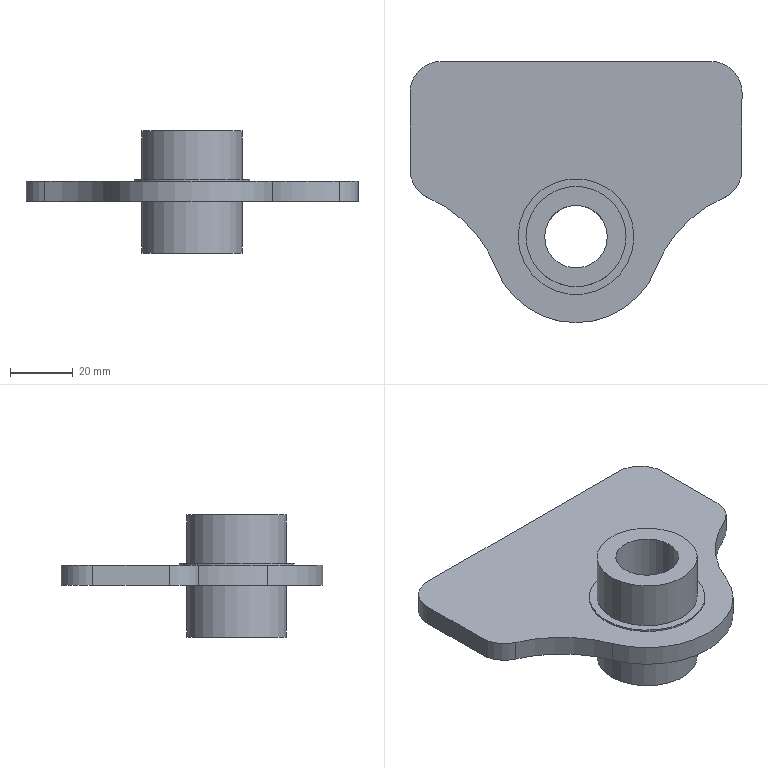CAM job | NX | 3-axis milling | part box 106 x 83.448 x 39 mm
Tools:
number,name,description,diameter,corner_radius,flute_length,length,flutes
1,D16-48-D16-100-3T-FINISH,D16-48-D16-100-3T,16.0,0.0,48.0,100.0,3
0,CHAMFER_D6-90DEG,倒角D6-90度,6.0,0.0,5.0,50.0,2
Operations:
program,operation,operation_type,tool,method,geometry_group,spindle_rpm,surface_speed,feed_per_tooth,feed_cut,feed_plunge,cut_length_mm,path_length_mm,cut_time_min,machine_time_min
A1,ADAPTIVE_MILLING,CavityMilling,D16-48-D16-100-3T-FINISH,METHOD,WORKPIECE_54,3000.0,150.0,0.2222,2000.0,100.0,1869.963,1923.663,0.935,0.9404
A1,PLANAR_MILL_1_COPY,PlanarMilling,D16-48-D16-100-3T-FINISH,METHOD,A-G54,3000.0,150.0,0.1111,1000.0,100.0,934.453,1018.253,0.9345,0.9428
A1,PLANAR_MILL,PlanarMilling,D16-48-D16-100-3T-FINISH,METHOD,A-G54,3000.0,150.0,0.1111,1000.0,100.0,131.268,185.268,0.1313,0.1367
A1,FLOOR_WALL,VolumeBased25DMillingOperation,D16-48-D16-100-3T-FINISH,METHOD,A-G54,3000.0,150.0,0.1111,1000.0,100.0,1066.072,1260.77,1.066,1.085
A1,PLANAR_MILL_1,PlanarMilling,D16-48-D16-100-3T-FINISH,METHOD,A-G54,3000.0,150.0,0.1111,1000.0,100.0,195.524,283.524,0.1955,0.2043
A1,PLANAR_MILL_4,PlanarMilling,D16-48-D16-100-3T-FINISH,METHOD,A-G54,3000.0,150.0,0.1111,1000.0,100.0,1188.74,1283.74,1.189,1.198
A1,PLANAR_MILL_4_COPY,PlanarMilling,D16-48-D16-100-3T-FINISH,METHOD,A-G54,3000.0,150.0,0.0333,300.0,100.0,40.146,174.146,0.1338,0.1472
A1,PLANAR_MILL_3,PlanarMilling,CHAMFER_D6-90DEG,METHOD,A-G54,3000.0,56.0,0.1,600.0,100.0,121.239,181.239,0.2021,0.2081
A1,PLANAR_MILL_3_COPY,PlanarMilling,CHAMFER_D6-90DEG,METHOD,A-G54,3000.0,56.0,0.1,600.0,100.0,65.321,125.321,0.1089,0.1149